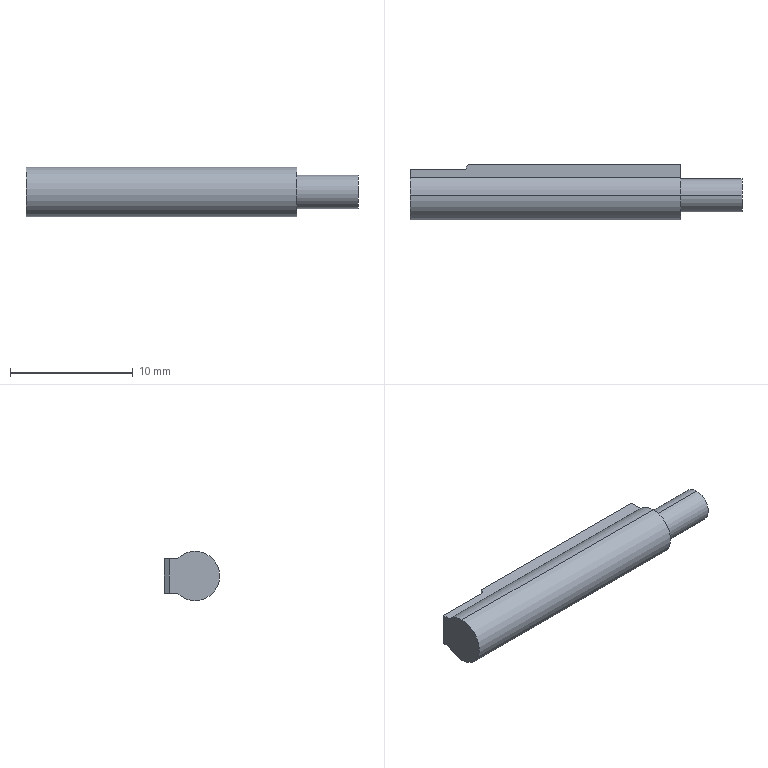Part | STEP file | _D-A93(CQ2_50).stp | 1 solid | 28 faces | box 27 x 4.5 x 4 mm | volume 337.66 mm3 | plane 19 | cylinder 9 | commonest cylinder face diameters 4 x3 2 x2 2.5 x2 2.7 x2